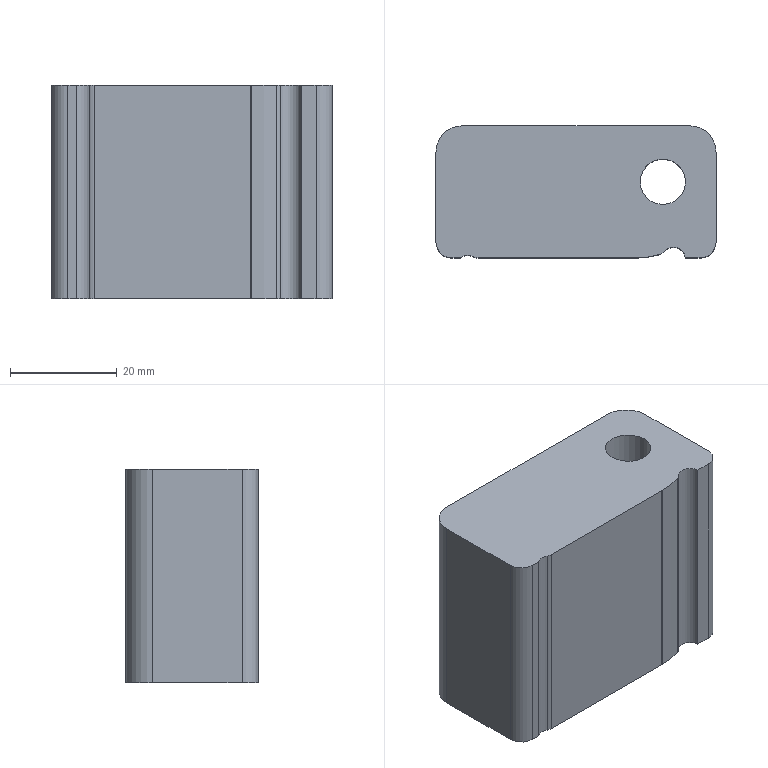Part | NX | features PS-39 2 | 1 solid | 22 faces | box 52.598 x 24.8 x 40 mm | volume 47765 mm3 | plane 10 | cylinder 10 | spline 2 | commonest cylinder face diameters 3.6 x2 4.4 x2 6 x2 10 x2 8.5 x1 14.5 x1
STEP:
#1=CARTESIAN_POINT('',(3907.497,-854.922,860.716));
#2=VERTEX_POINT('',#1);
#3=CARTESIAN_POINT('',(3907.495,-854.922,900.716));
#4=VERTEX_POINT('',#3);
#5=CARTESIAN_POINT('',(3907.495,-854.922,900.716));
#6=CARTESIAN_POINT('',(3907.495,-854.922,887.383));
#7=CARTESIAN_POINT('',(3907.495,-854.922,874.05));
#8=CARTESIAN_POINT('',(3907.495,-854.922,860.716));
#9=B_SPLINE_CURVE_WITH_KNOTS('',3,(#5,#6,#7,#8),.UNSPECIFIED.,.F.,.F.,(4,4),(-0.3333,1.),.UNSPECIFIED.);
#10=EDGE_CURVE('',#2,#4,#9,.F.);
#11=ORIENTED_EDGE('',*,*,#10,.T.);
#12=CARTESIAN_POINT('',(3878.173,-854.922,900.716));
#13=VERTEX_POINT('',#12);
#14=CARTESIAN_POINT('',(3873.236,-854.922,900.716));
#15=DIRECTION('',(-1.,0.,0.));
#16=VECTOR('',#15,1000.);
#17=LINE('',#14,#16);
#18=EDGE_CURVE('',#4,#13,#17,.T.);
#19=ORIENTED_EDGE('',*,*,#18,.T.);
#20=CARTESIAN_POINT('',(3878.173,-854.922,860.716));
#21=VERTEX_POINT('',#20);
#22=CARTESIAN_POINT('',(3878.173,-854.922,895.716));
#23=DIRECTION('',(0.,0.,1.));
#24=VECTOR('',#23,1000.);
#25=LINE('',#22,#24);
#26=EDGE_CURVE('',#13,#21,#25,.F.);
#27=ORIENTED_EDGE('',*,*,#26,.T.);
#28=CARTESIAN_POINT('',(3874.84,-854.922,860.716));
#29=DIRECTION('',(-1.,0.,0.));
#30=VECTOR('',#29,1000.);
#31=LINE('',#28,#30);
#32=EDGE_CURVE('',#21,#2,#31,.F.);
#33=ORIENTED_EDGE('',*,*,#32,.T.);
#34=EDGE_LOOP('',(#11,#19,#27,#33));
#35=FACE_BOUND('',#34,.T.);
#36=CARTESIAN_POINT('',(3874.84,-854.922,890.716));
#37=DIRECTION('',(0.,-1.,0.));
#38=DIRECTION('',(0.,0.,-1.));
#39=AXIS2_PLACEMENT_3D('',#36,#37,#38);
#40=PLANE('',#39);
#41=ADVANCED_FACE('',(#35),#40,.T.);
#42=CARTESIAN_POINT('',(3907.736,-854.922,860.716));
#43=VERTEX_POINT('',#42);
#44=CARTESIAN_POINT('',(3907.736,-854.922,900.716));
#45=VERTEX_POINT('',#44);
#46=CARTESIAN_POINT('',(3907.736,-854.922,895.716));
#47=DIRECTION('',(0.,0.,-1.));
#48=VECTOR('',#47,1000.);
#49=LINE('',#46,#48);
#50=EDGE_CURVE('',#43,#45,#49,.F.);
#51=ORIENTED_EDGE('',*,*,#50,.T.);
#52=CARTESIAN_POINT('',(3907.684,-854.922,900.716));
#53=VERTEX_POINT('',#52);
#54=CARTESIAN_POINT('',(3873.236,-854.922,900.716));
#55=DIRECTION('',(-1.,0.,0.));
#56=VECTOR('',#55,1000.);
#57=LINE('',#54,#56);
#58=EDGE_CURVE('',#45,#53,#57,.T.);
#59=ORIENTED_EDGE('',*,*,#58,.T.);
#60=CARTESIAN_POINT('',(3907.684,-854.922,860.716));
#61=VERTEX_POINT('',#60);
#62=CARTESIAN_POINT('',(3907.684,-854.922,895.716));
#63=DIRECTION('',(0.,0.,-1.));
#64=VECTOR('',#63,1000.);
#65=LINE('',#62,#64);
#66=EDGE_CURVE('',#53,#61,#65,.T.);
#67=ORIENTED_EDGE('',*,*,#66,.T.);
#68=CARTESIAN_POINT('',(3874.84,-854.922,860.716));
#69=DIRECTION('',(-1.,0.,0.));
#70=VECTOR('',#69,1000.);
#71=LINE('',#68,#70);
#72=EDGE_CURVE('',#61,#43,#71,.F.);
#73=ORIENTED_EDGE('',*,*,#72,.T.);
#74=EDGE_LOOP('',(#51,#59,#67,#73));
#75=FACE_BOUND('',#74,.T.);
#76=CARTESIAN_POINT('',(3874.84,-854.922,890.716));
#77=DIRECTION('',(0.,-1.,0.));
#78=DIRECTION('',(0.,0.,-1.));
#79=AXIS2_PLACEMENT_3D('',#76,#77,#78);
#80=PLANE('',#79);
#81=ADVANCED_FACE('',(#75),#80,.T.);
#82=CARTESIAN_POINT('',(3919.835,-854.922,900.716));
#83=VERTEX_POINT('',#82);
#84=CARTESIAN_POINT('',(3917.027,-854.922,900.716));
#85=VERTEX_POINT('',#84);
#86=CARTESIAN_POINT('',(3873.236,-854.922,900.716));
#87=DIRECTION('',(-1.,0.,0.));
#88=VECTOR('',#87,1000.);
#89=LINE('',#86,#88);
#90=EDGE_CURVE('',#83,#85,#89,.T.);
#91=ORIENTED_EDGE('',*,*,#90,.T.);
#92=CARTESIAN_POINT('',(3917.027,-854.922,860.716));
#93=VERTEX_POINT('',#92);
#94=CARTESIAN_POINT('',(3917.027,-854.922,935.716));
#95=DIRECTION('',(0.,0.,-1.));
#96=VECTOR('',#95,1000.);
#97=LINE('',#94,#96);
#98=EDGE_CURVE('',#85,#93,#97,.T.);
#99=ORIENTED_EDGE('',*,*,#98,.T.);
#100=CARTESIAN_POINT('',(3919.835,-854.922,860.716));
#101=VERTEX_POINT('',#100);
#102=CARTESIAN_POINT('',(3874.84,-854.922,860.716));
#103=DIRECTION('',(-1.,0.,0.));
#104=VECTOR('',#103,1000.);
#105=LINE('',#102,#104);
#106=EDGE_CURVE('',#93,#101,#105,.F.);
#107=ORIENTED_EDGE('',*,*,#106,.T.);
#108=CARTESIAN_POINT('',(3919.835,-854.922,890.716));
#109=DIRECTION('',(0.,0.,-1.));
#110=VECTOR('',#109,1000.);
#111=LINE('',#108,#110);
#112=EDGE_CURVE('',#83,#101,#111,.T.);
#113=ORIENTED_EDGE('',*,*,#112,.F.);
#114=EDGE_LOOP('',(#91,#99,#107,#113));
#115=FACE_BOUND('',#114,.T.);
#116=CARTESIAN_POINT('',(3874.84,-854.922,890.716));
#117=DIRECTION('',(0.,-1.,0.));
#118=DIRECTION('',(0.,0.,-1.));
#119=AXIS2_PLACEMENT_3D('',#116,#117,#118);
#120=PLANE('',#119);
#121=ADVANCED_FACE('',(#115),#120,.T.);
#122=CARTESIAN_POINT('',(3874.84,-854.922,860.716));
#123=VERTEX_POINT('',#122);
#124=CARTESIAN_POINT('',(3874.84,-854.922,900.716));
#125=VERTEX_POINT('',#124);
#126=CARTESIAN_POINT('',(3874.84,-854.922,935.716));
#127=DIRECTION('',(0.,0.,-1.));
#128=VECTOR('',#127,1000.);
#129=LINE('',#126,#128);
#130=EDGE_CURVE('',#123,#125,#129,.F.);
#131=ORIENTED_EDGE('',*,*,#130,.T.);
#132=CARTESIAN_POINT('',(3873.236,-854.922,900.716));
#133=VERTEX_POINT('',#132);
#134=CARTESIAN_POINT('',(3873.236,-854.922,900.716));
#135=DIRECTION('',(-1.,0.,0.));
#136=VECTOR('',#135,1000.);
#137=LINE('',#134,#136);
#138=EDGE_CURVE('',#125,#133,#137,.T.);
#139=ORIENTED_EDGE('',*,*,#138,.T.);
#140=CARTESIAN_POINT('',(3873.236,-854.922,860.716));
#141=VERTEX_POINT('',#140);
#142=CARTESIAN_POINT('',(3873.236,-854.922,890.716));
#143=DIRECTION('',(0.,0.,-1.));
#144=VECTOR('',#143,1000.);
#145=LINE('',#142,#144);
#146=EDGE_CURVE('',#133,#141,#145,.T.);
#147=ORIENTED_EDGE('',*,*,#146,.T.);
#148=CARTESIAN_POINT('',(3874.84,-854.922,860.716));
#149=DIRECTION('',(-1.,0.,0.));
#150=VECTOR('',#149,1000.);
#151=LINE('',#148,#150);
#152=EDGE_CURVE('',#141,#123,#151,.F.);
#153=ORIENTED_EDGE('',*,*,#152,.T.);
#154=EDGE_LOOP('',(#131,#139,#147,#153));
#155=FACE_BOUND('',#154,.T.);
#156=CARTESIAN_POINT('',(3874.84,-854.922,890.716));
#157=DIRECTION('',(0.,-1.,0.));
#158=DIRECTION('',(0.,0.,-1.));
#159=AXIS2_PLACEMENT_3D('',#156,#157,#158);
#160=PLANE('',#159);
#161=ADVANCED_FACE('',(#155),#160,.T.);
#162=CARTESIAN_POINT('',(3870.236,-851.922,860.716));
#163=VERTEX_POINT('',#162);
#164=CARTESIAN_POINT('',(3873.236,-851.922,860.716));
#165=DIRECTION('',(0.,0.,-1.));
#166=DIRECTION('',(1.,0.,0.));
#167=AXIS2_PLACEMENT_3D('',#164,#165,#166);
#168=CIRCLE('',#167,3.);
#169=EDGE_CURVE('',#163,#141,#168,.F.);
#170=ORIENTED_EDGE('',*,*,#169,.T.);
#171=ORIENTED_EDGE('',*,*,#146,.F.);
#172=CARTESIAN_POINT('',(3870.236,-851.922,900.716));
#173=VERTEX_POINT('',#172);
#174=CARTESIAN_POINT('',(3873.236,-851.922,900.716));
#175=DIRECTION('',(0.,0.,-1.));
#176=DIRECTION('',(-1.,0.,0.));
#177=AXIS2_PLACEMENT_3D('',#174,#175,#176);
#178=CIRCLE('',#177,3.);
#179=EDGE_CURVE('',#133,#173,#178,.T.);
#180=ORIENTED_EDGE('',*,*,#179,.T.);
#181=CARTESIAN_POINT('',(3870.236,-851.922,890.716));
#182=DIRECTION('',(0.,0.,-1.));
#183=VECTOR('',#182,1000.);
#184=LINE('',#181,#183);
#185=EDGE_CURVE('',#173,#163,#184,.T.);
#186=ORIENTED_EDGE('',*,*,#185,.T.);
#187=EDGE_LOOP('',(#170,#171,#180,#186));
#188=FACE_BOUND('',#187,.T.);
#189=CARTESIAN_POINT('',(3873.236,-851.922,890.716));
#190=DIRECTION('',(0.,0.,-1.));
#191=DIRECTION('',(-1.,0.,0.));
#192=AXIS2_PLACEMENT_3D('',#189,#190,#191);
#193=CYLINDRICAL_SURFACE('',#192,3.);
#194=ADVANCED_FACE('',(#188),#193,.T.);
#195=CARTESIAN_POINT('',(3870.236,-835.122,860.716));
#196=VERTEX_POINT('',#195);
#197=CARTESIAN_POINT('',(3870.236,-851.922,860.716));
#198=DIRECTION('',(0.,1.,0.));
#199=VECTOR('',#198,1000.);
#200=LINE('',#197,#199);
#201=EDGE_CURVE('',#196,#163,#200,.F.);
#202=ORIENTED_EDGE('',*,*,#201,.T.);
#203=ORIENTED_EDGE('',*,*,#185,.F.);
#204=CARTESIAN_POINT('',(3870.236,-835.122,900.716));
#205=VERTEX_POINT('',#204);
#206=CARTESIAN_POINT('',(3870.236,-851.922,900.716));
#207=DIRECTION('',(0.,1.,0.));
#208=VECTOR('',#207,1000.);
#209=LINE('',#206,#208);
#210=EDGE_CURVE('',#173,#205,#209,.T.);
#211=ORIENTED_EDGE('',*,*,#210,.T.);
#212=CARTESIAN_POINT('',(3870.236,-835.122,890.716));
#213=DIRECTION('',(0.,0.,-1.));
#214=VECTOR('',#213,1000.);
#215=LINE('',#212,#214);
#216=EDGE_CURVE('',#205,#196,#215,.T.);
#217=ORIENTED_EDGE('',*,*,#216,.T.);
#218=EDGE_LOOP('',(#202,#203,#211,#217));
#219=FACE_BOUND('',#218,.T.);
#220=CARTESIAN_POINT('',(3870.236,-851.922,890.716));
#221=DIRECTION('',(-1.,0.,0.));
#222=DIRECTION('',(0.,0.,1.));
#223=AXIS2_PLACEMENT_3D('',#220,#221,#222);
#224=PLANE('',#223);
#225=ADVANCED_FACE('',(#219),#224,.T.);
#226=CARTESIAN_POINT('',(3875.236,-830.122,860.716));
#227=VERTEX_POINT('',#226);
#228=CARTESIAN_POINT('',(3875.236,-835.122,860.716));
#229=DIRECTION('',(0.,0.,-1.));
#230=DIRECTION('',(1.,0.,0.));
#231=AXIS2_PLACEMENT_3D('',#228,#229,#230);
#232=CIRCLE('',#231,5.);
#233=EDGE_CURVE('',#227,#196,#232,.F.);
#234=ORIENTED_EDGE('',*,*,#233,.T.);
#235=ORIENTED_EDGE('',*,*,#216,.F.);
#236=CARTESIAN_POINT('',(3875.236,-830.122,900.716));
#237=VERTEX_POINT('',#236);
#238=CARTESIAN_POINT('',(3875.236,-835.122,900.716));
#239=DIRECTION('',(0.,0.,-1.));
#240=DIRECTION('',(-1.,0.,0.));
#241=AXIS2_PLACEMENT_3D('',#238,#239,#240);
#242=CIRCLE('',#241,5.);
#243=EDGE_CURVE('',#205,#237,#242,.T.);
#244=ORIENTED_EDGE('',*,*,#243,.T.);
#245=CARTESIAN_POINT('',(3875.236,-830.122,890.716));
#246=DIRECTION('',(0.,0.,-1.));
#247=VECTOR('',#246,1000.);
#248=LINE('',#245,#247);
#249=EDGE_CURVE('',#237,#227,#248,.T.);
#250=ORIENTED_EDGE('',*,*,#249,.T.);
#251=EDGE_LOOP('',(#234,#235,#244,#250));
#252=FACE_BOUND('',#251,.T.);
#253=CARTESIAN_POINT('',(3875.236,-835.122,890.716));
#254=DIRECTION('',(0.,0.,-1.));
#255=DIRECTION('',(-1.,0.,0.));
#256=AXIS2_PLACEMENT_3D('',#253,#254,#255);
#257=CYLINDRICAL_SURFACE('',#256,5.);
#258=ADVANCED_FACE('',(#252),#257,.T.);
#259=CARTESIAN_POINT('',(3917.835,-830.122,860.716));
#260=VERTEX_POINT('',#259);
#261=CARTESIAN_POINT('',(3875.236,-830.122,860.716));
#262=DIRECTION('',(1.,0.,0.));
#263=VECTOR('',#262,1000.);
#264=LINE('',#261,#263);
#265=EDGE_CURVE('',#260,#227,#264,.F.);
#266=ORIENTED_EDGE('',*,*,#265,.T.);
#267=ORIENTED_EDGE('',*,*,#249,.F.);
#268=CARTESIAN_POINT('',(3917.835,-830.122,900.716));
#269=VERTEX_POINT('',#268);
#270=CARTESIAN_POINT('',(3873.236,-830.122,900.716));
#271=DIRECTION('',(1.,0.,0.));
#272=VECTOR('',#271,1000.);
#273=LINE('',#270,#272);
#274=EDGE_CURVE('',#237,#269,#273,.T.);
#275=ORIENTED_EDGE('',*,*,#274,.T.);
#276=CARTESIAN_POINT('',(3917.835,-830.122,890.716));
#277=DIRECTION('',(0.,0.,-1.));
#278=VECTOR('',#277,1000.);
#279=LINE('',#276,#278);
#280=EDGE_CURVE('',#269,#260,#279,.T.);
#281=ORIENTED_EDGE('',*,*,#280,.T.);
#282=EDGE_LOOP('',(#266,#267,#275,#281));
#283=FACE_BOUND('',#282,.T.);
#284=CARTESIAN_POINT('',(3875.236,-830.122,890.716));
#285=DIRECTION('',(0.,1.,0.));
#286=DIRECTION('',(0.,0.,1.));
#287=AXIS2_PLACEMENT_3D('',#284,#285,#286);
#288=PLANE('',#287);
#289=ADVANCED_FACE('',(#283),#288,.T.);
#290=CARTESIAN_POINT('',(3922.835,-835.122,860.716));
#291=VERTEX_POINT('',#290);
#292=CARTESIAN_POINT('',(3917.835,-835.122,860.716));
#293=DIRECTION('',(0.,0.,-1.));
#294=DIRECTION('',(1.,0.,0.));
#295=AXIS2_PLACEMENT_3D('',#292,#293,#294);
#296=CIRCLE('',#295,5.);
#297=EDGE_CURVE('',#291,#260,#296,.F.);
#298=ORIENTED_EDGE('',*,*,#297,.T.);
#299=ORIENTED_EDGE('',*,*,#280,.F.);
#300=CARTESIAN_POINT('',(3922.835,-835.122,900.716));
#301=VERTEX_POINT('',#300);
#302=CARTESIAN_POINT('',(3917.835,-835.122,900.716));
#303=DIRECTION('',(0.,0.,-1.));
#304=DIRECTION('',(-1.,0.,0.));
#305=AXIS2_PLACEMENT_3D('',#302,#303,#304);
#306=CIRCLE('',#305,5.);
#307=EDGE_CURVE('',#269,#301,#306,.T.);
#308=ORIENTED_EDGE('',*,*,#307,.T.);
#309=CARTESIAN_POINT('',(3922.835,-835.122,890.716));
#310=DIRECTION('',(0.,0.,-1.));
#311=VECTOR('',#310,1000.);
#312=LINE('',#309,#311);
#313=EDGE_CURVE('',#301,#291,#312,.T.);
#314=ORIENTED_EDGE('',*,*,#313,.T.);
#315=EDGE_LOOP('',(#298,#299,#308,#314));
#316=FACE_BOUND('',#315,.T.);
#317=CARTESIAN_POINT('',(3917.835,-835.122,890.716));
#318=DIRECTION('',(0.,0.,-1.));
#319=DIRECTION('',(-1.,0.,0.));
#320=AXIS2_PLACEMENT_3D('',#317,#318,#319);
#321=CYLINDRICAL_SURFACE('',#320,5.);
#322=ADVANCED_FACE('',(#316),#321,.T.);
#323=CARTESIAN_POINT('',(3922.835,-851.922,860.716));
#324=VERTEX_POINT('',#323);
#325=CARTESIAN_POINT('',(3922.835,-835.122,860.716));
#326=DIRECTION('',(0.,-1.,0.));
#327=VECTOR('',#326,1000.);
#328=LINE('',#325,#327);
#329=EDGE_CURVE('',#324,#291,#328,.F.);
#330=ORIENTED_EDGE('',*,*,#329,.T.);
#331=ORIENTED_EDGE('',*,*,#313,.F.);
#332=CARTESIAN_POINT('',(3922.835,-851.922,900.716));
#333=VERTEX_POINT('',#332);
#334=CARTESIAN_POINT('',(3922.835,-851.922,900.716));
#335=DIRECTION('',(0.,-1.,0.));
#336=VECTOR('',#335,1000.);
#337=LINE('',#334,#336);
#338=EDGE_CURVE('',#301,#333,#337,.T.);
#339=ORIENTED_EDGE('',*,*,#338,.T.);
#340=CARTESIAN_POINT('',(3922.835,-851.922,890.716));
#341=DIRECTION('',(0.,0.,-1.));
#342=VECTOR('',#341,1000.);
#343=LINE('',#340,#342);
#344=EDGE_CURVE('',#333,#324,#343,.T.);
#345=ORIENTED_EDGE('',*,*,#344,.T.);
#346=EDGE_LOOP('',(#330,#331,#339,#345));
#347=FACE_BOUND('',#346,.T.);
#348=CARTESIAN_POINT('',(3922.835,-835.122,890.716));
#349=DIRECTION('',(1.,0.,0.));
#350=DIRECTION('',(0.,0.,-1.));
#351=AXIS2_PLACEMENT_3D('',#348,#349,#350);
#352=PLANE('',#351);
#353=ADVANCED_FACE('',(#347),#352,.T.);
#354=CARTESIAN_POINT('',(3919.835,-851.922,860.716));
#355=DIRECTION('',(0.,0.,-1.));
#356=DIRECTION('',(1.,0.,0.));
#357=AXIS2_PLACEMENT_3D('',#354,#355,#356);
#358=CIRCLE('',#357,3.);
#359=EDGE_CURVE('',#101,#324,#358,.F.);
#360=ORIENTED_EDGE('',*,*,#359,.T.);
#361=ORIENTED_EDGE('',*,*,#344,.F.);
#362=CARTESIAN_POINT('',(3919.835,-851.922,900.716));
#363=DIRECTION('',(0.,0.,-1.));
#364=DIRECTION('',(-1.,0.,0.));
#365=AXIS2_PLACEMENT_3D('',#362,#363,#364);
#366=CIRCLE('',#365,3.);
#367=EDGE_CURVE('',#333,#83,#366,.T.);
#368=ORIENTED_EDGE('',*,*,#367,.T.);
#369=ORIENTED_EDGE('',*,*,#112,.T.);
#370=EDGE_LOOP('',(#360,#361,#368,#369));
#371=FACE_BOUND('',#370,.T.);
#372=CARTESIAN_POINT('',(3919.835,-851.922,890.716));
#373=DIRECTION('',(0.,0.,-1.));
#374=DIRECTION('',(-1.,0.,0.));
#375=AXIS2_PLACEMENT_3D('',#372,#373,#374);
#376=CYLINDRICAL_SURFACE('',#375,3.);
#377=ADVANCED_FACE('',(#371),#376,.T.);
#378=CARTESIAN_POINT('',(3920.085,-840.639,860.716));
#379=VERTEX_POINT('',#378);
#380=CARTESIAN_POINT('',(3912.835,-840.639,860.716));
#381=DIRECTION('',(0.,0.,1.));
#382=DIRECTION('',(1.,0.,0.));
#383=AXIS2_PLACEMENT_3D('',#380,#381,#382);
#384=CIRCLE('',#383,7.25);
#385=EDGE_CURVE('',#379,#379,#384,.T.);
#386=ORIENTED_EDGE('',*,*,#385,.T.);
#387=EDGE_LOOP('',(#386));
#388=FACE_BOUND('',#387,.T.);
#389=CARTESIAN_POINT('',(3907.498,-854.921,860.716));
#390=CARTESIAN_POINT('',(3907.56,-854.921,860.716));
#391=CARTESIAN_POINT('',(3907.622,-854.922,860.716));
#392=CARTESIAN_POINT('',(3907.684,-854.922,860.716));
#393=B_SPLINE_CURVE_WITH_KNOTS('',3,(#389,#390,#391,#392),.UNSPECIFIED.,.F.,.F.,(4,4),(0.,1.),.UNSPECIFIED.);
#394=EDGE_CURVE('',#2,#61,#393,.T.);
#395=ORIENTED_EDGE('',*,*,#394,.F.);
#396=ORIENTED_EDGE('',*,*,#32,.F.);
#397=CARTESIAN_POINT('',(3877.301,-854.697,860.716));
#398=VERTEX_POINT('',#397);
#399=CARTESIAN_POINT('',(3878.173,-853.122,860.716));
#400=DIRECTION('',(0.,0.,-1.));
#401=DIRECTION('',(-1.,0.,0.));
#402=AXIS2_PLACEMENT_3D('',#399,#400,#401);
#403=CIRCLE('',#402,1.8);
#404=EDGE_CURVE('',#21,#398,#403,.T.);
#405=ORIENTED_EDGE('',*,*,#404,.T.);
#406=CARTESIAN_POINT('',(3876.236,-856.622,860.716));
#407=DIRECTION('',(0.,0.,-1.));
#408=DIRECTION('',(-1.,0.,0.));
#409=AXIS2_PLACEMENT_3D('',#406,#407,#408);
#410=CIRCLE('',#409,2.2);
#411=EDGE_CURVE('',#398,#123,#410,.F.);
#412=ORIENTED_EDGE('',*,*,#411,.T.);
#413=ORIENTED_EDGE('',*,*,#152,.F.);
#414=ORIENTED_EDGE('',*,*,#169,.F.);
#415=ORIENTED_EDGE('',*,*,#201,.F.);
#416=ORIENTED_EDGE('',*,*,#233,.F.);
#417=ORIENTED_EDGE('',*,*,#265,.F.);
#418=ORIENTED_EDGE('',*,*,#297,.F.);
#419=ORIENTED_EDGE('',*,*,#329,.F.);
#420=ORIENTED_EDGE('',*,*,#359,.F.);
#421=ORIENTED_EDGE('',*,*,#106,.F.);
#422=CARTESIAN_POINT('',(3913.158,-853.68,860.716));
#423=VERTEX_POINT('',#422);
#424=CARTESIAN_POINT('',(3914.835,-855.105,860.716));
#425=DIRECTION('',(0.,0.,-1.));
#426=DIRECTION('',(-1.,0.,0.));
#427=AXIS2_PLACEMENT_3D('',#424,#425,#426);
#428=CIRCLE('',#427,2.2);
#429=EDGE_CURVE('',#423,#93,#428,.T.);
#430=ORIENTED_EDGE('',*,*,#429,.F.);
#431=CARTESIAN_POINT('',(3912.314,-854.235,860.716));
#432=VERTEX_POINT('',#431);
#433=CARTESIAN_POINT('',(3911.787,-852.514,860.716));
#434=DIRECTION('',(0.,0.,-1.));
#435=DIRECTION('',(-1.,0.,0.));
#436=AXIS2_PLACEMENT_3D('',#433,#434,#435);
#437=CIRCLE('',#436,1.8);
#438=EDGE_CURVE('',#432,#423,#437,.F.);
#439=ORIENTED_EDGE('',*,*,#438,.F.);
#440=CARTESIAN_POINT('',(3907.736,-854.922,860.716));
#441=CARTESIAN_POINT('',(3909.286,-854.92,860.716));
#442=CARTESIAN_POINT('',(3910.831,-854.687,860.716));
#443=CARTESIAN_POINT('',(3912.314,-854.236,860.716));
#444=B_SPLINE_CURVE_WITH_KNOTS('',3,(#440,#441,#442,#443),.UNSPECIFIED.,.F.,.F.,(4,4),(0.,0.004647),.UNSPECIFIED.);
#445=EDGE_CURVE('',#43,#432,#444,.T.);
#446=ORIENTED_EDGE('',*,*,#445,.F.);
#447=ORIENTED_EDGE('',*,*,#72,.F.);
#448=EDGE_LOOP('',(#395,#396,#405,#412,#413,#414,#415,#416,#417,#418,#419,#420,#421,#430,#439,#446,#447));
#449=FACE_BOUND('',#448,.T.);
#450=CARTESIAN_POINT('',(3919.835,-851.922,860.716));
#451=DIRECTION('',(0.,0.,-1.));
#452=DIRECTION('',(-1.,0.,0.));
#453=AXIS2_PLACEMENT_3D('',#450,#451,#452);
#454=PLANE('',#453);
#455=ADVANCED_FACE('',(#388,#449),#454,.T.);
#456=CARTESIAN_POINT('',(3908.585,-840.639,900.716));
#457=VERTEX_POINT('',#456);
#458=CARTESIAN_POINT('',(3912.835,-840.639,900.716));
#459=DIRECTION('',(0.,0.,-1.));
#460=DIRECTION('',(-1.,0.,0.));
#461=AXIS2_PLACEMENT_3D('',#458,#459,#460);
#462=CIRCLE('',#461,4.25);
#463=EDGE_CURVE('',#457,#457,#462,.T.);
#464=ORIENTED_EDGE('',*,*,#463,.T.);
#465=EDGE_LOOP('',(#464));
#466=FACE_BOUND('',#465,.T.);
#467=ORIENTED_EDGE('',*,*,#18,.F.);
#468=CARTESIAN_POINT('',(3907.684,-854.922,900.716));
#469=CARTESIAN_POINT('',(3907.621,-854.922,900.716));
#470=CARTESIAN_POINT('',(3907.558,-854.921,900.716));
#471=CARTESIAN_POINT('',(3907.495,-854.921,900.716));
#472=B_SPLINE_CURVE_WITH_KNOTS('',3,(#468,#469,#470,#471),.UNSPECIFIED.,.F.,.F.,(4,4),(0.,0.0001886),.UNSPECIFIED.);
#473=EDGE_CURVE('',#53,#4,#472,.T.);
#474=ORIENTED_EDGE('',*,*,#473,.F.);
#475=ORIENTED_EDGE('',*,*,#58,.F.);
#476=CARTESIAN_POINT('',(3912.314,-854.236,900.716));
#477=VERTEX_POINT('',#476);
#478=CARTESIAN_POINT('',(3912.314,-854.236,900.716));
#479=CARTESIAN_POINT('',(3910.832,-854.687,900.716));
#480=CARTESIAN_POINT('',(3909.286,-854.92,900.716));
#481=CARTESIAN_POINT('',(3907.736,-854.922,900.716));
#482=B_SPLINE_CURVE_WITH_KNOTS('',3,(#478,#479,#480,#481),.UNSPECIFIED.,.F.,.F.,(4,4),(0.01978,0.02443),.UNSPECIFIED.);
#483=EDGE_CURVE('',#477,#45,#482,.T.);
#484=ORIENTED_EDGE('',*,*,#483,.F.);
#485=CARTESIAN_POINT('',(3913.158,-853.68,900.716));
#486=VERTEX_POINT('',#485);
#487=CARTESIAN_POINT('',(3911.787,-852.514,900.716));
#488=DIRECTION('',(0.,0.,-1.));
#489=DIRECTION('',(-1.,0.,0.));
#490=AXIS2_PLACEMENT_3D('',#487,#488,#489);
#491=CIRCLE('',#490,1.8);
#492=EDGE_CURVE('',#477,#486,#491,.F.);
#493=ORIENTED_EDGE('',*,*,#492,.T.);
#494=CARTESIAN_POINT('',(3914.835,-855.105,900.716));
#495=DIRECTION('',(0.,0.,-1.));
#496=DIRECTION('',(-1.,0.,0.));
#497=AXIS2_PLACEMENT_3D('',#494,#495,#496);
#498=CIRCLE('',#497,2.2);
#499=EDGE_CURVE('',#85,#486,#498,.F.);
#500=ORIENTED_EDGE('',*,*,#499,.F.);
#501=ORIENTED_EDGE('',*,*,#90,.F.);
#502=ORIENTED_EDGE('',*,*,#367,.F.);
#503=ORIENTED_EDGE('',*,*,#338,.F.);
#504=ORIENTED_EDGE('',*,*,#307,.F.);
#505=ORIENTED_EDGE('',*,*,#274,.F.);
#506=ORIENTED_EDGE('',*,*,#243,.F.);
#507=ORIENTED_EDGE('',*,*,#210,.F.);
#508=ORIENTED_EDGE('',*,*,#179,.F.);
#509=ORIENTED_EDGE('',*,*,#138,.F.);
#510=CARTESIAN_POINT('',(3877.301,-854.697,900.716));
#511=VERTEX_POINT('',#510);
#512=CARTESIAN_POINT('',(3876.236,-856.622,900.716));
#513=DIRECTION('',(0.,0.,-1.));
#514=DIRECTION('',(-1.,0.,0.));
#515=AXIS2_PLACEMENT_3D('',#512,#513,#514);
#516=CIRCLE('',#515,2.2);
#517=EDGE_CURVE('',#125,#511,#516,.T.);
#518=ORIENTED_EDGE('',*,*,#517,.T.);
#519=CARTESIAN_POINT('',(3878.173,-853.122,900.716));
#520=DIRECTION('',(0.,0.,-1.));
#521=DIRECTION('',(-1.,0.,0.));
#522=AXIS2_PLACEMENT_3D('',#519,#520,#521);
#523=CIRCLE('',#522,1.8);
#524=EDGE_CURVE('',#13,#511,#523,.T.);
#525=ORIENTED_EDGE('',*,*,#524,.F.);
#526=EDGE_LOOP('',(#467,#474,#475,#484,#493,#500,#501,#502,#503,#504,#505,#506,#507,#508,#509,#518,#525));
#527=FACE_BOUND('',#526,.T.);
#528=CARTESIAN_POINT('',(3873.236,-851.922,900.716));
#529=DIRECTION('',(0.,0.,-1.));
#530=DIRECTION('',(-1.,0.,0.));
#531=AXIS2_PLACEMENT_3D('',#528,#529,#530);
#532=PLANE('',#531);
#533=ADVANCED_FACE('',(#466,#527),#532,.F.);
#534=CARTESIAN_POINT('',(3913.158,-853.68,935.716));
#535=DIRECTION('',(0.,0.,-1.));
#536=VECTOR('',#535,1000.);
#537=LINE('',#534,#536);
#538=EDGE_CURVE('',#423,#486,#537,.F.);
#539=ORIENTED_EDGE('',*,*,#538,.T.);
#540=ORIENTED_EDGE('',*,*,#492,.F.);
#541=CARTESIAN_POINT('',(3912.314,-854.235,860.716));
#542=CARTESIAN_POINT('',(3912.314,-854.235,874.05));
#543=CARTESIAN_POINT('',(3912.314,-854.235,887.383));
#544=CARTESIAN_POINT('',(3912.314,-854.235,900.716));
#545=B_SPLINE_CURVE_WITH_KNOTS('',3,(#541,#542,#543,#544),.UNSPECIFIED.,.F.,.F.,(4,4),(0.0625,0.5625),.UNSPECIFIED.);
#546=EDGE_CURVE('',#432,#477,#545,.T.);
#547=ORIENTED_EDGE('',*,*,#546,.F.);
#548=ORIENTED_EDGE('',*,*,#438,.T.);
#549=EDGE_LOOP('',(#539,#540,#547,#548));
#550=FACE_BOUND('',#549,.T.);
#551=CARTESIAN_POINT('',(3911.787,-852.514,935.716));
#552=DIRECTION('',(0.,0.,-1.));
#553=DIRECTION('',(-1.,0.,0.));
#554=AXIS2_PLACEMENT_3D('',#551,#552,#553);
#555=CYLINDRICAL_SURFACE('',#554,1.8);
#556=ADVANCED_FACE('',(#550),#555,.T.);
#557=ORIENTED_EDGE('',*,*,#98,.F.);
#558=ORIENTED_EDGE('',*,*,#499,.T.);
#559=ORIENTED_EDGE('',*,*,#538,.F.);
#560=ORIENTED_EDGE('',*,*,#429,.T.);
#561=EDGE_LOOP('',(#557,#558,#559,#560));
#562=FACE_BOUND('',#561,.T.);
#563=CARTESIAN_POINT('',(3914.835,-855.105,935.716));
#564=DIRECTION('',(0.,0.,-1.));
#565=DIRECTION('',(-1.,0.,0.));
#566=AXIS2_PLACEMENT_3D('',#563,#564,#565);
#567=CYLINDRICAL_SURFACE('',#566,2.2);
#568=ADVANCED_FACE('',(#562),#567,.F.);
#569=ORIENTED_EDGE('',*,*,#445,.T.);
#570=ORIENTED_EDGE('',*,*,#546,.T.);
#571=ORIENTED_EDGE('',*,*,#483,.T.);
#572=ORIENTED_EDGE('',*,*,#50,.F.);
#573=EDGE_LOOP('',(#569,#570,#571,#572));
#574=FACE_BOUND('',#573,.T.);
#575=CARTESIAN_POINT('',(3912.314,-854.236,900.716));
#576=CARTESIAN_POINT('',(3912.314,-854.236,860.716));
#577=CARTESIAN_POINT('',(3910.833,-854.687,900.716));
#578=CARTESIAN_POINT('',(3910.833,-854.687,860.716));
#579=CARTESIAN_POINT('',(3909.29,-854.92,900.716));
#580=CARTESIAN_POINT('',(3909.29,-854.92,860.716));
#581=CARTESIAN_POINT('',(3907.736,-854.922,900.716));
#582=CARTESIAN_POINT('',(3907.736,-854.922,860.716));
#583=B_SPLINE_SURFACE_WITH_KNOTS('',3,1,((#575,#576),(#577,#578),(#579,#580),(#581,#582)),.SURF_OF_LINEAR_EXTRUSION.,.F.,.F.,.F.,(4,4),(2,2),(0.3963,0.9707),(0.,1.),.PIECEWISE_BEZIER_KNOTS.);
#584=ADVANCED_FACE('',(#574),#583,.T.);
#585=ORIENTED_EDGE('',*,*,#404,.F.);
#586=ORIENTED_EDGE('',*,*,#26,.F.);
#587=ORIENTED_EDGE('',*,*,#524,.T.);
#588=CARTESIAN_POINT('',(3877.301,-854.697,935.716));
#589=DIRECTION('',(0.,0.,-1.));
#590=VECTOR('',#589,1000.);
#591=LINE('',#588,#590);
#592=EDGE_CURVE('',#398,#511,#591,.F.);
#593=ORIENTED_EDGE('',*,*,#592,.F.);
#594=EDGE_LOOP('',(#585,#586,#587,#593));
#595=FACE_BOUND('',#594,.T.);
#596=CARTESIAN_POINT('',(3878.173,-853.122,935.716));
#597=DIRECTION('',(0.,0.,-1.));
#598=DIRECTION('',(-1.,0.,0.));
#599=AXIS2_PLACEMENT_3D('',#596,#597,#598);
#600=CYLINDRICAL_SURFACE('',#599,1.8);
#601=ADVANCED_FACE('',(#595),#600,.T.);
#602=ORIENTED_EDGE('',*,*,#411,.F.);
#603=ORIENTED_EDGE('',*,*,#592,.T.);
#604=ORIENTED_EDGE('',*,*,#517,.F.);
#605=ORIENTED_EDGE('',*,*,#130,.F.);
#606=EDGE_LOOP('',(#602,#603,#604,#605));
#607=FACE_BOUND('',#606,.T.);
#608=CARTESIAN_POINT('',(3876.236,-856.622,935.716));
#609=DIRECTION('',(0.,0.,-1.));
#610=DIRECTION('',(-1.,0.,0.));
#611=AXIS2_PLACEMENT_3D('',#608,#609,#610);
#612=CYLINDRICAL_SURFACE('',#611,2.2);
#613=ADVANCED_FACE('',(#607),#612,.F.);
#614=ORIENTED_EDGE('',*,*,#394,.T.);
#615=ORIENTED_EDGE('',*,*,#66,.F.);
#616=ORIENTED_EDGE('',*,*,#473,.T.);
#617=ORIENTED_EDGE('',*,*,#10,.F.);
#618=EDGE_LOOP('',(#614,#615,#616,#617));
#619=FACE_BOUND('',#618,.T.);
#620=CARTESIAN_POINT('',(3907.684,-854.922,900.716));
#621=CARTESIAN_POINT('',(3907.684,-854.922,860.716));
#622=CARTESIAN_POINT('',(3907.621,-854.922,900.716));
#623=CARTESIAN_POINT('',(3907.621,-854.922,860.716));
#624=CARTESIAN_POINT('',(3907.558,-854.921,900.716));
#625=CARTESIAN_POINT('',(3907.558,-854.921,860.716));
#626=CARTESIAN_POINT('',(3907.494,-854.921,900.716));
#627=CARTESIAN_POINT('',(3907.494,-854.921,860.716));
#628=B_SPLINE_SURFACE_WITH_KNOTS('',3,1,((#620,#621),(#622,#623),(#624,#625),(#626,#627)),.SURF_OF_LINEAR_EXTRUSION.,.F.,.F.,.F.,(4,4),(2,2),(0.9771,1.),(0.,1.),.PIECEWISE_BEZIER_KNOTS.);
#629=ADVANCED_FACE('',(#619),#628,.T.);
#630=CARTESIAN_POINT('',(3917.085,-840.639,871.716));
#631=VERTEX_POINT('',#630);
#632=CARTESIAN_POINT('',(3912.835,-840.639,871.716));
#633=DIRECTION('',(0.,0.,1.));
#634=DIRECTION('',(1.,0.,0.));
#635=AXIS2_PLACEMENT_3D('',#632,#633,#634);
#636=CIRCLE('',#635,4.25);
#637=EDGE_CURVE('',#631,#631,#636,.T.);
#638=ORIENTED_EDGE('',*,*,#637,.F.);
#639=EDGE_LOOP('',(#638));
#640=FACE_BOUND('',#639,.T.);
#641=ORIENTED_EDGE('',*,*,#463,.F.);
#642=EDGE_LOOP('',(#641));
#643=FACE_BOUND('',#642,.T.);
#644=CARTESIAN_POINT('',(3912.835,-840.639,860.716));
#645=DIRECTION('',(0.,0.,1.));
#646=DIRECTION('',(1.,0.,0.));
#647=AXIS2_PLACEMENT_3D('',#644,#645,#646);
#648=CYLINDRICAL_SURFACE('',#647,4.25);
#649=ADVANCED_FACE('',(#640,#643),#648,.F.);
#650=ORIENTED_EDGE('',*,*,#637,.T.);
#651=EDGE_LOOP('',(#650));
#652=FACE_BOUND('',#651,.T.);
#653=CARTESIAN_POINT('',(3920.085,-840.639,871.716));
#654=VERTEX_POINT('',#653);
#655=CARTESIAN_POINT('',(3912.835,-840.639,871.716));
#656=DIRECTION('',(0.,0.,-1.));
#657=DIRECTION('',(1.,0.,0.));
#658=AXIS2_PLACEMENT_3D('',#655,#656,#657);
#659=CIRCLE('',#658,7.25);
#660=EDGE_CURVE('',#654,#654,#659,.F.);
#661=ORIENTED_EDGE('',*,*,#660,.F.);
#662=EDGE_LOOP('',(#661));
#663=FACE_BOUND('',#662,.T.);
#664=CARTESIAN_POINT('',(3912.835,-840.639,871.716));
#665=DIRECTION('',(0.,0.,1.));
#666=DIRECTION('',(1.,0.,0.));
#667=AXIS2_PLACEMENT_3D('',#664,#665,#666);
#668=PLANE('',#667);
#669=ADVANCED_FACE('',(#652,#663),#668,.F.);
#670=ORIENTED_EDGE('',*,*,#660,.T.);
#671=EDGE_LOOP('',(#670));
#672=FACE_BOUND('',#671,.T.);
#673=ORIENTED_EDGE('',*,*,#385,.F.);
#674=EDGE_LOOP('',(#673));
#675=FACE_BOUND('',#674,.T.);
#676=CARTESIAN_POINT('',(3912.835,-840.639,860.716));
#677=DIRECTION('',(0.,0.,1.));
#678=DIRECTION('',(1.,0.,0.));
#679=AXIS2_PLACEMENT_3D('',#676,#677,#678);
#680=CYLINDRICAL_SURFACE('',#679,7.25);
#681=ADVANCED_FACE('',(#672,#675),#680,.F.);
#682=CLOSED_SHELL('',(#41,#81,#121,#161,#194,#225,#258,#289,#322,#353,#377,#455,#533,#556,#568,#584,#601,#613,#629,#649,#669,#681));
#683=MANIFOLD_SOLID_BREP('',#682);
#684=(LENGTH_UNIT()NAMED_UNIT(*)SI_UNIT(.MILLI.,.METRE.));
#685=UNCERTAINTY_MEASURE_WITH_UNIT(LENGTH_MEASURE(0.05108),#684,'','');
#686=(NAMED_UNIT(*)PLANE_ANGLE_UNIT()SI_UNIT($,.RADIAN.));
#687=(NAMED_UNIT(*)SI_UNIT($,.STERADIAN.)SOLID_ANGLE_UNIT());
#688=(GEOMETRIC_REPRESENTATION_CONTEXT(3)GLOBAL_UNCERTAINTY_ASSIGNED_CONTEXT((#685))GLOBAL_UNIT_ASSIGNED_CONTEXT((#684,#686,#687))REPRESENTATION_CONTEXT('',''));
#689=ADVANCED_BREP_SHAPE_REPRESENTATION('',(#683),#688);